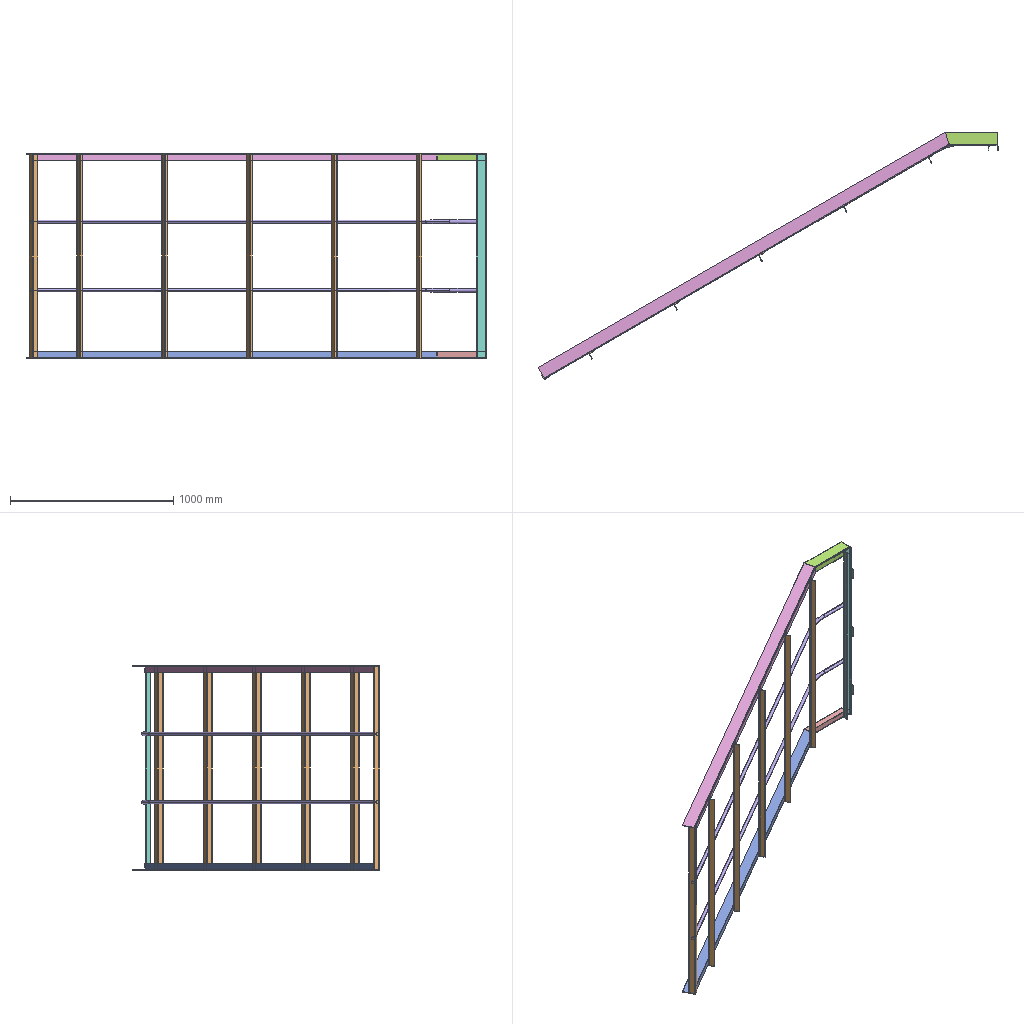Assembly | SolidWorks | 7 different items | 13 placed | box 2817 x 1515 x 1250 mm
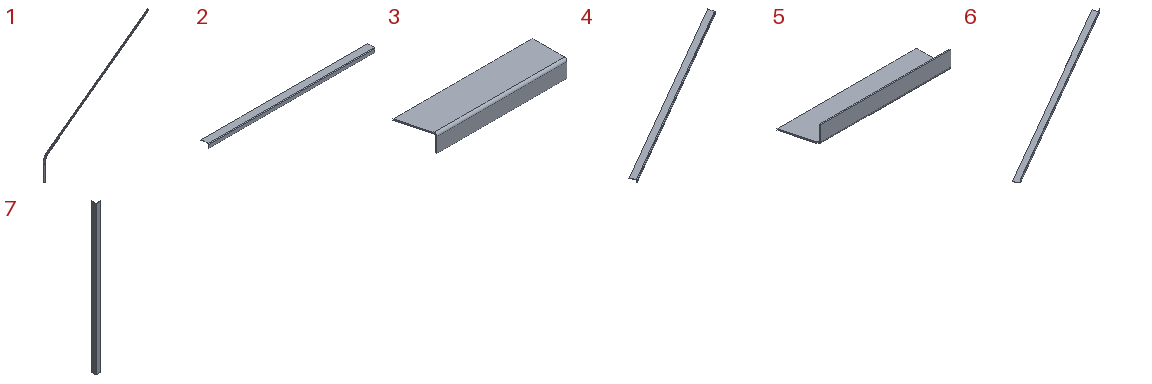Parts list (item | quantity | size | volume | features):
1 | x2 | 22 x 1453 x 2786 mm | 397136 mm3 | features Sweep 1
2 | x1 | 1250 x 60 x 30 mm | 350614 mm3 | features EdgeFlange 1, Fillet 1, FlatPattern 1, ICE 1, SMBaseFlange 1, SheetMetal 1
3 | x1 | 321.436 x 80 x 40 mm | 106111 mm3 | features EdgeFlange 1, FlatPattern 1, ICE 1, SMBaseFlange 1, SheetMetal 1
4 | x1 | 2517 x 1510 x 40 mm | 989838 mm3 | features EdgeFlange 1, FlatPattern 1, ICE 1, SMBaseFlange 1, SheetMetal 1
5 | x1 | 321.436 x 80 x 40 mm | 106111 mm3 | features EdgeFlange 1, FlatPattern 1, ICE 1, SMBaseFlange 1, SheetMetal 1
6 | x1 | 2517 x 1510 x 40 mm | 989838 mm3 | features EdgeFlange 1, FlatPattern 1, ICE 1, SMBaseFlange 1, SheetMetal 1
7 | x6 | 40 x 40 x 1250 mm | 385753 mm3 | features ICE 1, LibraryFeature 1
Mates (type | each side: item.copy, entity, surface, feature):
Coincident | 5.1 face plane Base-Flange1 | 6.1 face plane Base-Flange1 | 2 times
Coincident | 5.1 edge | 6.1 edge
Coincident | 5.1 face plane Edge-Flange1 | 3.1 face plane Edge-Flange1 | 2 times
DistanceDim | 3.1 face plane Base-Flange1 | 5.1 face plane Base-Flange1
Coincident | 3.1 face plane Base-Flange1 | 4.1 face plane Base-Flange1 | 2 times
Coincident | 3.1 edge | 4.1 edge
Coincident | 3.1 face plane Edge-Flange1 | 2.1 face plane Base-Flange1
Coincident | 3.1 face plane Edge-Flange1 | 2.1 face plane Edge-Flange1
Coincident | 5.1 face plane Base-Flange1 | 2.1 face plane Base-Flange1
Coincident | 4.1 face plane Edge-Flange1 | 7.1 face plane Boss-Extrude1
Coincident | 4.1 face plane Base-Flange1 | 7.1 face plane Boss-Extrude1
DistanceDim | 7.1 face plane Boss-Extrude1 | 3.1 vertex
Coincident | 4.1 face plane Base-Flange1 | 7.2 face plane Boss-Extrude1 | 2 times
Coincident | 4.1 face plane Edge-Flange1 | 7.2 face plane Boss-Extrude1
DistanceDim | 2.1 plane | 1.1 plane
Coincident | 7.2 face plane Boss-Extrude1 | 1.1 face plane Sweep1
Tangent | 7.3 face plane Boss-Extrude1 | 1.1 face cylinder Sweep1